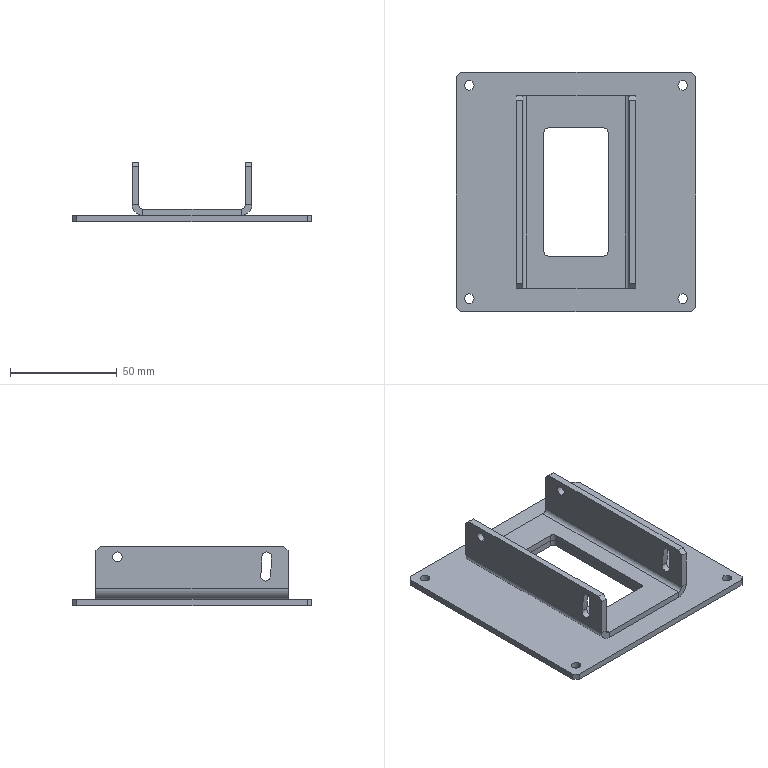Part | SolidWorks | features Chamfer 2, FlatPattern 2, HoleWzd 2, ICE 2, SMBaseFlange 2, SheetMetal 2 | 2 solids | 74 faces | box 112 x 112 x 28 mm | volume 52364 mm3 | plane 40 | cylinder 34 | commonest cylinder face diameters 4.5 x18 4 x10 10 x2 135.5 x2 144.5 x2